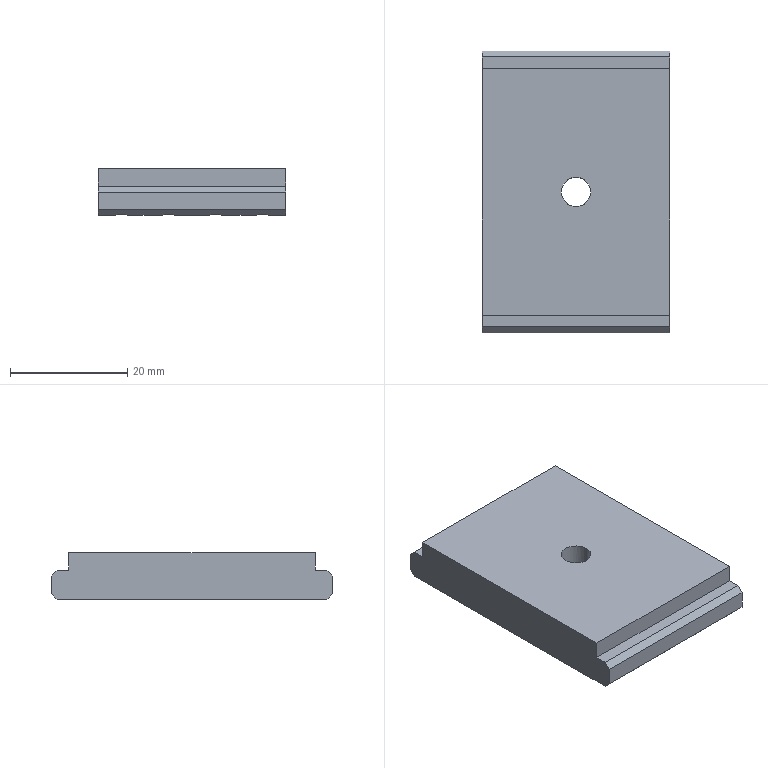Part | SolidWorks | features BaseBody 1, HoleWzd 1 | 1 solid | 43 faces | box 32 x 48 x 8 mm | volume 8228 mm3 | plane 33 | cylinder 10 | commonest cylinder face diameters 4.5 x8 5 x2
STEP:
#1=CARTESIAN_POINT('',(-1.75,-1.785,4.));
#2=VERTEX_POINT('',#1);
#3=CARTESIAN_POINT('',(-2.5,0.,4.));
#4=VERTEX_POINT('',#3);
#5=CARTESIAN_POINT('',(0.,0.,4.));
#6=DIRECTION('',(0.,0.,-1.));
#7=DIRECTION('',(-1.,0.,0.));
#8=AXIS2_PLACEMENT_3D('',#5,#6,#7);
#9=CIRCLE('',#8,2.5);
#10=EDGE_CURVE('',#2,#4,#9,.T.);
#11=ORIENTED_EDGE('',*,*,#10,.T.);
#12=CARTESIAN_POINT('',(-2.5,0.,8.));
#13=VERTEX_POINT('',#12);
#14=CARTESIAN_POINT('',(-2.5,0.,8.));
#15=DIRECTION('',(0.,0.,1.));
#16=VECTOR('',#15,1000.);
#17=LINE('',#14,#16);
#18=EDGE_CURVE('',#4,#13,#17,.T.);
#19=ORIENTED_EDGE('',*,*,#18,.T.);
#20=CARTESIAN_POINT('',(2.5,0.,8.));
#21=VERTEX_POINT('',#20);
#22=CARTESIAN_POINT('',(0.,0.,8.));
#23=DIRECTION('',(0.,0.,1.));
#24=DIRECTION('',(1.,0.,0.));
#25=AXIS2_PLACEMENT_3D('',#22,#23,#24);
#26=CIRCLE('',#25,2.5);
#27=EDGE_CURVE('',#13,#21,#26,.T.);
#28=ORIENTED_EDGE('',*,*,#27,.T.);
#29=CARTESIAN_POINT('',(2.5,0.,4.));
#30=VERTEX_POINT('',#29);
#31=CARTESIAN_POINT('',(2.5,0.,8.));
#32=DIRECTION('',(0.,0.,1.));
#33=VECTOR('',#32,1000.);
#34=LINE('',#31,#33);
#35=EDGE_CURVE('',#30,#21,#34,.T.);
#36=ORIENTED_EDGE('',*,*,#35,.F.);
#37=CARTESIAN_POINT('',(1.75,-1.785,4.));
#38=VERTEX_POINT('',#37);
#39=CARTESIAN_POINT('',(0.,0.,4.));
#40=DIRECTION('',(0.,0.,-1.));
#41=DIRECTION('',(-1.,0.,0.));
#42=AXIS2_PLACEMENT_3D('',#39,#40,#41);
#43=CIRCLE('',#42,2.5);
#44=EDGE_CURVE('',#30,#38,#43,.T.);
#45=ORIENTED_EDGE('',*,*,#44,.T.);
#46=CARTESIAN_POINT('',(1.75,-1.785,0.));
#47=VERTEX_POINT('',#46);
#48=CARTESIAN_POINT('',(1.75,-1.785,8.));
#49=DIRECTION('',(0.,0.,-1.));
#50=VECTOR('',#49,1000.);
#51=LINE('',#48,#50);
#52=EDGE_CURVE('',#38,#47,#51,.T.);
#53=ORIENTED_EDGE('',*,*,#52,.T.);
#54=CARTESIAN_POINT('',(-1.75,-1.785,0.));
#55=VERTEX_POINT('',#54);
#56=CARTESIAN_POINT('',(0.,0.,0.));
#57=DIRECTION('',(0.,0.,1.));
#58=DIRECTION('',(1.,0.,0.));
#59=AXIS2_PLACEMENT_3D('',#56,#57,#58);
#60=CIRCLE('',#59,2.5);
#61=EDGE_CURVE('',#55,#47,#60,.T.);
#62=ORIENTED_EDGE('',*,*,#61,.F.);
#63=CARTESIAN_POINT('',(-1.75,-1.785,8.));
#64=DIRECTION('',(0.,0.,-1.));
#65=VECTOR('',#64,1000.);
#66=LINE('',#63,#65);
#67=EDGE_CURVE('',#2,#55,#66,.T.);
#68=ORIENTED_EDGE('',*,*,#67,.F.);
#69=EDGE_LOOP('',(#11,#19,#28,#36,#45,#53,#62,#68));
#70=FACE_OUTER_BOUND('',#69,.T.);
#71=CARTESIAN_POINT('',(0.,0.,8.));
#72=DIRECTION('',(0.,0.,1.));
#73=DIRECTION('',(1.,0.,0.));
#74=AXIS2_PLACEMENT_3D('',#71,#72,#73);
#75=CYLINDRICAL_SURFACE('',#74,2.5);
#76=ADVANCED_FACE('',(#70),#75,.F.);
#77=CARTESIAN_POINT('',(1.75,1.785,0.));
#78=VERTEX_POINT('',#77);
#79=CARTESIAN_POINT('',(1.75,1.785,4.));
#80=VERTEX_POINT('',#79);
#81=CARTESIAN_POINT('',(1.75,1.785,8.));
#82=DIRECTION('',(0.,0.,1.));
#83=VECTOR('',#82,1000.);
#84=LINE('',#81,#83);
#85=EDGE_CURVE('',#78,#80,#84,.T.);
#86=ORIENTED_EDGE('',*,*,#85,.F.);
#87=CARTESIAN_POINT('',(1.75,21.,0.));
#88=VERTEX_POINT('',#87);
#89=CARTESIAN_POINT('',(1.75,21.,0.));
#90=DIRECTION('',(0.,-1.,0.));
#91=VECTOR('',#90,1000.);
#92=LINE('',#89,#91);
#93=EDGE_CURVE('',#88,#78,#92,.T.);
#94=ORIENTED_EDGE('',*,*,#93,.F.);
#95=CARTESIAN_POINT('',(1.75,21.,4.));
#96=VERTEX_POINT('',#95);
#97=CARTESIAN_POINT('',(1.75,21.,4.));
#98=DIRECTION('',(0.,0.,-1.));
#99=VECTOR('',#98,1000.);
#100=LINE('',#97,#99);
#101=EDGE_CURVE('',#96,#88,#100,.T.);
#102=ORIENTED_EDGE('',*,*,#101,.F.);
#103=CARTESIAN_POINT('',(1.75,21.,4.));
#104=DIRECTION('',(0.,-1.,0.));
#105=VECTOR('',#104,1000.);
#106=LINE('',#103,#105);
#107=EDGE_CURVE('',#96,#80,#106,.T.);
#108=ORIENTED_EDGE('',*,*,#107,.T.);
#109=EDGE_LOOP('',(#86,#94,#102,#108));
#110=FACE_OUTER_BOUND('',#109,.T.);
#111=CARTESIAN_POINT('',(1.75,21.,4.));
#112=DIRECTION('',(1.,0.,0.));
#113=DIRECTION('',(0.,1.,0.));
#114=AXIS2_PLACEMENT_3D('',#111,#112,#113);
#115=PLANE('',#114);
#116=ADVANCED_FACE('',(#110),#115,.T.);
#117=ORIENTED_EDGE('',*,*,#93,.T.);
#118=CARTESIAN_POINT('',(-1.75,1.785,0.));
#119=VERTEX_POINT('',#118);
#120=CARTESIAN_POINT('',(0.,0.,0.));
#121=DIRECTION('',(0.,0.,1.));
#122=DIRECTION('',(1.,0.,0.));
#123=AXIS2_PLACEMENT_3D('',#120,#121,#122);
#124=CIRCLE('',#123,2.5);
#125=EDGE_CURVE('',#78,#119,#124,.T.);
#126=ORIENTED_EDGE('',*,*,#125,.T.);
#127=CARTESIAN_POINT('',(-1.75,21.,0.));
#128=VERTEX_POINT('',#127);
#129=CARTESIAN_POINT('',(-1.75,21.,0.));
#130=DIRECTION('',(0.,-1.,0.));
#131=VECTOR('',#130,1000.);
#132=LINE('',#129,#131);
#133=EDGE_CURVE('',#128,#119,#132,.T.);
#134=ORIENTED_EDGE('',*,*,#133,.F.);
#135=CARTESIAN_POINT('',(-2.969,23.,0.));
#136=VERTEX_POINT('',#135);
#137=CARTESIAN_POINT('',(-4.,21.,0.));
#138=DIRECTION('',(0.,0.,-1.));
#139=DIRECTION('',(-1.,0.,0.));
#140=AXIS2_PLACEMENT_3D('',#137,#138,#139);
#141=CIRCLE('',#140,2.25);
#142=EDGE_CURVE('',#136,#128,#141,.T.);
#143=ORIENTED_EDGE('',*,*,#142,.F.);
#144=CARTESIAN_POINT('',(2.969,23.,0.));
#145=VERTEX_POINT('',#144);
#146=CARTESIAN_POINT('',(0.,23.,0.));
#147=DIRECTION('',(1.,0.,0.));
#148=VECTOR('',#147,1000.);
#149=LINE('',#146,#148);
#150=EDGE_CURVE('',#136,#145,#149,.T.);
#151=ORIENTED_EDGE('',*,*,#150,.T.);
#152=CARTESIAN_POINT('',(4.,21.,0.));
#153=DIRECTION('',(0.,0.,1.));
#154=DIRECTION('',(1.,0.,0.));
#155=AXIS2_PLACEMENT_3D('',#152,#153,#154);
#156=CIRCLE('',#155,2.25);
#157=EDGE_CURVE('',#145,#88,#156,.T.);
#158=ORIENTED_EDGE('',*,*,#157,.T.);
#159=EDGE_LOOP('',(#117,#126,#134,#143,#151,#158));
#160=FACE_OUTER_BOUND('',#159,.T.);
#161=CARTESIAN_POINT('',(0.,0.,0.));
#162=DIRECTION('',(0.,0.,1.));
#163=DIRECTION('',(1.,0.,0.));
#164=AXIS2_PLACEMENT_3D('',#161,#162,#163);
#165=PLANE('',#164);
#166=ADVANCED_FACE('',(#160),#165,.F.);
#167=ORIENTED_EDGE('',*,*,#133,.T.);
#168=CARTESIAN_POINT('',(-1.75,1.785,4.));
#169=VERTEX_POINT('',#168);
#170=CARTESIAN_POINT('',(-1.75,1.785,8.));
#171=DIRECTION('',(0.,0.,1.));
#172=VECTOR('',#171,1000.);
#173=LINE('',#170,#172);
#174=EDGE_CURVE('',#119,#169,#173,.T.);
#175=ORIENTED_EDGE('',*,*,#174,.T.);
#176=CARTESIAN_POINT('',(-1.75,21.,4.));
#177=VERTEX_POINT('',#176);
#178=CARTESIAN_POINT('',(-1.75,21.,4.));
#179=DIRECTION('',(0.,-1.,0.));
#180=VECTOR('',#179,1000.);
#181=LINE('',#178,#180);
#182=EDGE_CURVE('',#177,#169,#181,.T.);
#183=ORIENTED_EDGE('',*,*,#182,.F.);
#184=CARTESIAN_POINT('',(-1.75,21.,4.));
#185=DIRECTION('',(0.,0.,-1.));
#186=VECTOR('',#185,1000.);
#187=LINE('',#184,#186);
#188=EDGE_CURVE('',#177,#128,#187,.T.);
#189=ORIENTED_EDGE('',*,*,#188,.T.);
#190=EDGE_LOOP('',(#167,#175,#183,#189));
#191=FACE_OUTER_BOUND('',#190,.T.);
#192=CARTESIAN_POINT('',(-1.75,21.,4.));
#193=DIRECTION('',(1.,0.,0.));
#194=DIRECTION('',(0.,1.,0.));
#195=AXIS2_PLACEMENT_3D('',#192,#193,#194);
#196=PLANE('',#195);
#197=ADVANCED_FACE('',(#191),#196,.F.);
#198=CARTESIAN_POINT('',(13.031,-23.,0.));
#199=VERTEX_POINT('',#198);
#200=CARTESIAN_POINT('',(10.969,-23.,0.));
#201=VERTEX_POINT('',#200);
#202=CARTESIAN_POINT('',(13.031,-23.,0.));
#203=CARTESIAN_POINT('',(12.371,-23.34,0.34));
#204=CARTESIAN_POINT('',(11.629,-23.34,0.34));
#205=CARTESIAN_POINT('',(10.969,-23.,0.));
#206=(BOUNDED_CURVE()B_SPLINE_CURVE(3,(#202,#203,#204,#205),.UNSPECIFIED.,.F.,.F.)B_SPLINE_CURVE_WITH_KNOTS((4,4),(2.666,3.617),.UNSPECIFIED.)CURVE()GEOMETRIC_REPRESENTATION_ITEM()RATIONAL_B_SPLINE_CURVE((1.,0.9259,0.9259,1.))REPRESENTATION_ITEM(''));
#207=EDGE_CURVE('',#199,#201,#206,.T.);
#208=ORIENTED_EDGE('',*,*,#207,.F.);
#209=CARTESIAN_POINT('',(16.,-23.,0.));
#210=VERTEX_POINT('',#209);
#211=CARTESIAN_POINT('',(0.,-23.,0.));
#212=DIRECTION('',(-1.,0.,0.));
#213=VECTOR('',#212,1000.);
#214=LINE('',#211,#213);
#215=EDGE_CURVE('',#210,#199,#214,.T.);
#216=ORIENTED_EDGE('',*,*,#215,.F.);
#217=CARTESIAN_POINT('',(16.,-24.,1.));
#218=VERTEX_POINT('',#217);
#219=CARTESIAN_POINT('',(16.,-24.,1.));
#220=DIRECTION('',(0.,0.7071,-0.7071));
#221=VECTOR('',#220,1000.);
#222=LINE('',#219,#221);
#223=EDGE_CURVE('',#218,#210,#222,.T.);
#224=ORIENTED_EDGE('',*,*,#223,.F.);
#225=CARTESIAN_POINT('',(-16.,-24.,1.));
#226=VERTEX_POINT('',#225);
#227=CARTESIAN_POINT('',(-16.,-24.,1.));
#228=DIRECTION('',(1.,0.,0.));
#229=VECTOR('',#228,1000.);
#230=LINE('',#227,#229);
#231=EDGE_CURVE('',#226,#218,#230,.T.);
#232=ORIENTED_EDGE('',*,*,#231,.F.);
#233=CARTESIAN_POINT('',(-16.,-23.,0.));
#234=VERTEX_POINT('',#233);
#235=CARTESIAN_POINT('',(-16.,-24.,1.));
#236=DIRECTION('',(0.,-0.7071,0.7071));
#237=VECTOR('',#236,1000.);
#238=LINE('',#235,#237);
#239=EDGE_CURVE('',#234,#226,#238,.T.);
#240=ORIENTED_EDGE('',*,*,#239,.F.);
#241=CARTESIAN_POINT('',(-13.031,-23.,0.));
#242=VERTEX_POINT('',#241);
#243=CARTESIAN_POINT('',(0.,-23.,0.));
#244=DIRECTION('',(-1.,0.,0.));
#245=VECTOR('',#244,1000.);
#246=LINE('',#243,#245);
#247=EDGE_CURVE('',#242,#234,#246,.T.);
#248=ORIENTED_EDGE('',*,*,#247,.F.);
#249=CARTESIAN_POINT('',(-10.969,-23.,0.));
#250=VERTEX_POINT('',#249);
#251=CARTESIAN_POINT('',(-10.969,-23.,0.));
#252=CARTESIAN_POINT('',(-11.629,-23.34,0.34));
#253=CARTESIAN_POINT('',(-12.371,-23.34,0.34));
#254=CARTESIAN_POINT('',(-13.031,-23.,0.));
#255=(BOUNDED_CURVE()B_SPLINE_CURVE(3,(#251,#252,#253,#254),.UNSPECIFIED.,.F.,.T.)B_SPLINE_CURVE_WITH_KNOTS((4,4),(2.666,3.617),.UNSPECIFIED.)CURVE()GEOMETRIC_REPRESENTATION_ITEM()RATIONAL_B_SPLINE_CURVE((1.,0.9259,0.9259,1.))REPRESENTATION_ITEM(''));
#256=EDGE_CURVE('',#250,#242,#255,.T.);
#257=ORIENTED_EDGE('',*,*,#256,.F.);
#258=CARTESIAN_POINT('',(-5.031,-23.,0.));
#259=VERTEX_POINT('',#258);
#260=CARTESIAN_POINT('',(0.,-23.,0.));
#261=DIRECTION('',(-1.,0.,0.));
#262=VECTOR('',#261,1000.);
#263=LINE('',#260,#262);
#264=EDGE_CURVE('',#259,#250,#263,.T.);
#265=ORIENTED_EDGE('',*,*,#264,.F.);
#266=CARTESIAN_POINT('',(-2.969,-23.,0.));
#267=VERTEX_POINT('',#266);
#268=CARTESIAN_POINT('',(-2.969,-23.,0.));
#269=CARTESIAN_POINT('',(-3.629,-23.34,0.34));
#270=CARTESIAN_POINT('',(-4.371,-23.34,0.34));
#271=CARTESIAN_POINT('',(-5.031,-23.,0.));
#272=(BOUNDED_CURVE()B_SPLINE_CURVE(3,(#268,#269,#270,#271),.UNSPECIFIED.,.F.,.F.)B_SPLINE_CURVE_WITH_KNOTS((4,4),(2.666,3.617),.UNSPECIFIED.)CURVE()GEOMETRIC_REPRESENTATION_ITEM()RATIONAL_B_SPLINE_CURVE((1.,0.9259,0.9259,1.))REPRESENTATION_ITEM(''));
#273=EDGE_CURVE('',#267,#259,#272,.T.);
#274=ORIENTED_EDGE('',*,*,#273,.F.);
#275=CARTESIAN_POINT('',(2.969,-23.,0.));
#276=VERTEX_POINT('',#275);
#277=CARTESIAN_POINT('',(0.,-23.,0.));
#278=DIRECTION('',(-1.,0.,0.));
#279=VECTOR('',#278,1000.);
#280=LINE('',#277,#279);
#281=EDGE_CURVE('',#276,#267,#280,.T.);
#282=ORIENTED_EDGE('',*,*,#281,.F.);
#283=CARTESIAN_POINT('',(5.031,-23.,0.));
#284=VERTEX_POINT('',#283);
#285=CARTESIAN_POINT('',(5.031,-23.,0.));
#286=CARTESIAN_POINT('',(4.371,-23.34,0.34));
#287=CARTESIAN_POINT('',(3.629,-23.34,0.34));
#288=CARTESIAN_POINT('',(2.969,-23.,0.));
#289=(BOUNDED_CURVE()B_SPLINE_CURVE(3,(#285,#286,#287,#288),.UNSPECIFIED.,.F.,.F.)B_SPLINE_CURVE_WITH_KNOTS((4,4),(2.666,3.617),.UNSPECIFIED.)CURVE()GEOMETRIC_REPRESENTATION_ITEM()RATIONAL_B_SPLINE_CURVE((1.,0.9259,0.9259,1.))REPRESENTATION_ITEM(''));
#290=EDGE_CURVE('',#284,#276,#289,.T.);
#291=ORIENTED_EDGE('',*,*,#290,.F.);
#292=CARTESIAN_POINT('',(0.,-23.,0.));
#293=DIRECTION('',(-1.,0.,0.));
#294=VECTOR('',#293,1000.);
#295=LINE('',#292,#294);
#296=EDGE_CURVE('',#201,#284,#295,.T.);
#297=ORIENTED_EDGE('',*,*,#296,.F.);
#298=EDGE_LOOP('',(#208,#216,#224,#232,#240,#248,#257,#265,#274,#282,#291,#297));
#299=FACE_OUTER_BOUND('',#298,.T.);
#300=CARTESIAN_POINT('',(-16.,-24.,1.));
#301=DIRECTION('',(0.,0.7071,0.7071));
#302=DIRECTION('',(1.,0.,0.));
#303=AXIS2_PLACEMENT_3D('',#300,#301,#302);
#304=PLANE('',#303);
#305=ADVANCED_FACE('',(#299),#304,.F.);
#306=CARTESIAN_POINT('',(-16.,-24.,4.));
#307=VERTEX_POINT('',#306);
#308=CARTESIAN_POINT('',(-16.,-23.,5.));
#309=VERTEX_POINT('',#308);
#310=CARTESIAN_POINT('',(-16.,-23.,5.));
#311=DIRECTION('',(0.,0.7071,0.7071));
#312=VECTOR('',#311,1000.);
#313=LINE('',#310,#312);
#314=EDGE_CURVE('',#307,#309,#313,.T.);
#315=ORIENTED_EDGE('',*,*,#314,.F.);
#316=CARTESIAN_POINT('',(16.,-24.,4.));
#317=VERTEX_POINT('',#316);
#318=CARTESIAN_POINT('',(-16.,-24.,4.));
#319=DIRECTION('',(-1.,0.,0.));
#320=VECTOR('',#319,1000.);
#321=LINE('',#318,#320);
#322=EDGE_CURVE('',#317,#307,#321,.T.);
#323=ORIENTED_EDGE('',*,*,#322,.F.);
#324=CARTESIAN_POINT('',(16.,-23.,5.));
#325=VERTEX_POINT('',#324);
#326=CARTESIAN_POINT('',(16.,-23.,5.));
#327=DIRECTION('',(0.,-0.7071,-0.7071));
#328=VECTOR('',#327,1000.);
#329=LINE('',#326,#328);
#330=EDGE_CURVE('',#325,#317,#329,.T.);
#331=ORIENTED_EDGE('',*,*,#330,.F.);
#332=CARTESIAN_POINT('',(-23.,-23.,5.));
#333=DIRECTION('',(1.,0.,0.));
#334=VECTOR('',#333,1000.);
#335=LINE('',#332,#334);
#336=EDGE_CURVE('',#309,#325,#335,.T.);
#337=ORIENTED_EDGE('',*,*,#336,.F.);
#338=EDGE_LOOP('',(#315,#323,#331,#337));
#339=FACE_OUTER_BOUND('',#338,.T.);
#340=CARTESIAN_POINT('',(-23.,-23.,5.));
#341=DIRECTION('',(0.,0.7071,-0.7071));
#342=DIRECTION('',(-1.,0.,0.));
#343=AXIS2_PLACEMENT_3D('',#340,#341,#342);
#344=PLANE('',#343);
#345=ADVANCED_FACE('',(#339),#344,.F.);
#346=CARTESIAN_POINT('',(-13.031,23.,0.));
#347=VERTEX_POINT('',#346);
#348=CARTESIAN_POINT('',(-10.969,23.,0.));
#349=VERTEX_POINT('',#348);
#350=CARTESIAN_POINT('',(-13.031,23.,0.));
#351=CARTESIAN_POINT('',(-12.371,23.34,0.34));
#352=CARTESIAN_POINT('',(-11.629,23.34,0.34));
#353=CARTESIAN_POINT('',(-10.969,23.,0.));
#354=(BOUNDED_CURVE()B_SPLINE_CURVE(3,(#350,#351,#352,#353),.UNSPECIFIED.,.F.,.F.)B_SPLINE_CURVE_WITH_KNOTS((4,4),(5.807,6.759),.UNSPECIFIED.)CURVE()GEOMETRIC_REPRESENTATION_ITEM()RATIONAL_B_SPLINE_CURVE((1.,0.9259,0.9259,1.))REPRESENTATION_ITEM(''));
#355=EDGE_CURVE('',#347,#349,#354,.T.);
#356=ORIENTED_EDGE('',*,*,#355,.F.);
#357=CARTESIAN_POINT('',(-16.,23.,0.));
#358=VERTEX_POINT('',#357);
#359=CARTESIAN_POINT('',(0.,23.,0.));
#360=DIRECTION('',(1.,0.,0.));
#361=VECTOR('',#360,1000.);
#362=LINE('',#359,#361);
#363=EDGE_CURVE('',#358,#347,#362,.T.);
#364=ORIENTED_EDGE('',*,*,#363,.F.);
#365=CARTESIAN_POINT('',(-16.,24.,1.));
#366=VERTEX_POINT('',#365);
#367=CARTESIAN_POINT('',(-16.,24.,1.));
#368=DIRECTION('',(0.,-0.7071,-0.7071));
#369=VECTOR('',#368,1000.);
#370=LINE('',#367,#369);
#371=EDGE_CURVE('',#366,#358,#370,.T.);
#372=ORIENTED_EDGE('',*,*,#371,.F.);
#373=CARTESIAN_POINT('',(16.,24.,1.));
#374=VERTEX_POINT('',#373);
#375=CARTESIAN_POINT('',(-16.,24.,1.));
#376=DIRECTION('',(-1.,0.,0.));
#377=VECTOR('',#376,1000.);
#378=LINE('',#375,#377);
#379=EDGE_CURVE('',#374,#366,#378,.T.);
#380=ORIENTED_EDGE('',*,*,#379,.F.);
#381=CARTESIAN_POINT('',(16.,23.,0.));
#382=VERTEX_POINT('',#381);
#383=CARTESIAN_POINT('',(16.,24.,1.));
#384=DIRECTION('',(0.,0.7071,0.7071));
#385=VECTOR('',#384,1000.);
#386=LINE('',#383,#385);
#387=EDGE_CURVE('',#382,#374,#386,.T.);
#388=ORIENTED_EDGE('',*,*,#387,.F.);
#389=CARTESIAN_POINT('',(13.031,23.,0.));
#390=VERTEX_POINT('',#389);
#391=CARTESIAN_POINT('',(0.,23.,0.));
#392=DIRECTION('',(1.,0.,0.));
#393=VECTOR('',#392,1000.);
#394=LINE('',#391,#393);
#395=EDGE_CURVE('',#390,#382,#394,.T.);
#396=ORIENTED_EDGE('',*,*,#395,.F.);
#397=CARTESIAN_POINT('',(10.969,23.,0.));
#398=VERTEX_POINT('',#397);
#399=CARTESIAN_POINT('',(10.969,23.,0.));
#400=CARTESIAN_POINT('',(11.629,23.34,0.34));
#401=CARTESIAN_POINT('',(12.371,23.34,0.34));
#402=CARTESIAN_POINT('',(13.031,23.,0.));
#403=(BOUNDED_CURVE()B_SPLINE_CURVE(3,(#399,#400,#401,#402),.UNSPECIFIED.,.F.,.F.)B_SPLINE_CURVE_WITH_KNOTS((4,4),(5.807,6.759),.UNSPECIFIED.)CURVE()GEOMETRIC_REPRESENTATION_ITEM()RATIONAL_B_SPLINE_CURVE((1.,0.9259,0.9259,1.))REPRESENTATION_ITEM(''));
#404=EDGE_CURVE('',#398,#390,#403,.T.);
#405=ORIENTED_EDGE('',*,*,#404,.F.);
#406=CARTESIAN_POINT('',(5.031,23.,0.));
#407=VERTEX_POINT('',#406);
#408=CARTESIAN_POINT('',(0.,23.,0.));
#409=DIRECTION('',(1.,0.,0.));
#410=VECTOR('',#409,1000.);
#411=LINE('',#408,#410);
#412=EDGE_CURVE('',#407,#398,#411,.T.);
#413=ORIENTED_EDGE('',*,*,#412,.F.);
#414=CARTESIAN_POINT('',(2.969,23.,0.));
#415=CARTESIAN_POINT('',(3.629,23.34,0.34));
#416=CARTESIAN_POINT('',(4.371,23.34,0.34));
#417=CARTESIAN_POINT('',(5.031,23.,0.));
#418=(BOUNDED_CURVE()B_SPLINE_CURVE(3,(#414,#415,#416,#417),.UNSPECIFIED.,.F.,.F.)B_SPLINE_CURVE_WITH_KNOTS((4,4),(5.807,6.759),.UNSPECIFIED.)CURVE()GEOMETRIC_REPRESENTATION_ITEM()RATIONAL_B_SPLINE_CURVE((1.,0.9259,0.9259,1.))REPRESENTATION_ITEM(''));
#419=EDGE_CURVE('',#145,#407,#418,.T.);
#420=ORIENTED_EDGE('',*,*,#419,.F.);
#421=ORIENTED_EDGE('',*,*,#150,.F.);
#422=CARTESIAN_POINT('',(-5.031,23.,0.));
#423=VERTEX_POINT('',#422);
#424=CARTESIAN_POINT('',(-5.031,23.,0.));
#425=CARTESIAN_POINT('',(-4.371,23.34,0.34));
#426=CARTESIAN_POINT('',(-3.629,23.34,0.34));
#427=CARTESIAN_POINT('',(-2.969,23.,0.));
#428=(BOUNDED_CURVE()B_SPLINE_CURVE(3,(#424,#425,#426,#427),.UNSPECIFIED.,.F.,.F.)B_SPLINE_CURVE_WITH_KNOTS((4,4),(5.807,6.759),.UNSPECIFIED.)CURVE()GEOMETRIC_REPRESENTATION_ITEM()RATIONAL_B_SPLINE_CURVE((1.,0.9259,0.9259,1.))REPRESENTATION_ITEM(''));
#429=EDGE_CURVE('',#423,#136,#428,.T.);
#430=ORIENTED_EDGE('',*,*,#429,.F.);
#431=CARTESIAN_POINT('',(0.,23.,0.));
#432=DIRECTION('',(1.,0.,0.));
#433=VECTOR('',#432,1000.);
#434=LINE('',#431,#433);
#435=EDGE_CURVE('',#349,#423,#434,.T.);
#436=ORIENTED_EDGE('',*,*,#435,.F.);
#437=EDGE_LOOP('',(#356,#364,#372,#380,#388,#396,#405,#413,#420,#421,#430,#436));
#438=FACE_OUTER_BOUND('',#437,.T.);
#439=CARTESIAN_POINT('',(-16.,24.,1.));
#440=DIRECTION('',(0.,-0.7071,0.7071));
#441=DIRECTION('',(-1.,0.,0.));
#442=AXIS2_PLACEMENT_3D('',#439,#440,#441);
#443=PLANE('',#442);
#444=ADVANCED_FACE('',(#438),#443,.F.);
#445=CARTESIAN_POINT('',(-16.,23.,5.));
#446=VERTEX_POINT('',#445);
#447=CARTESIAN_POINT('',(-16.,24.,4.));
#448=VERTEX_POINT('',#447);
#449=CARTESIAN_POINT('',(-16.,24.,4.));
#450=DIRECTION('',(0.,0.7071,-0.7071));
#451=VECTOR('',#450,1000.);
#452=LINE('',#449,#451);
#453=EDGE_CURVE('',#446,#448,#452,.T.);
#454=ORIENTED_EDGE('',*,*,#453,.F.);
#455=CARTESIAN_POINT('',(16.,23.,5.));
#456=VERTEX_POINT('',#455);
#457=CARTESIAN_POINT('',(-23.,23.,5.));
#458=DIRECTION('',(-1.,0.,0.));
#459=VECTOR('',#458,1000.);
#460=LINE('',#457,#459);
#461=EDGE_CURVE('',#456,#446,#460,.T.);
#462=ORIENTED_EDGE('',*,*,#461,.F.);
#463=CARTESIAN_POINT('',(16.,24.,4.));
#464=VERTEX_POINT('',#463);
#465=CARTESIAN_POINT('',(16.,24.,4.));
#466=DIRECTION('',(0.,-0.7071,0.7071));
#467=VECTOR('',#466,1000.);
#468=LINE('',#465,#467);
#469=EDGE_CURVE('',#464,#456,#468,.T.);
#470=ORIENTED_EDGE('',*,*,#469,.F.);
#471=CARTESIAN_POINT('',(-16.,24.,4.));
#472=DIRECTION('',(1.,0.,0.));
#473=VECTOR('',#472,1000.);
#474=LINE('',#471,#473);
#475=EDGE_CURVE('',#448,#464,#474,.T.);
#476=ORIENTED_EDGE('',*,*,#475,.F.);
#477=EDGE_LOOP('',(#454,#462,#470,#476));
#478=FACE_OUTER_BOUND('',#477,.T.);
#479=CARTESIAN_POINT('',(-16.,24.,4.));
#480=DIRECTION('',(0.,-0.7071,-0.7071));
#481=DIRECTION('',(0.,-0.7071,0.7071));
#482=AXIS2_PLACEMENT_3D('',#479,#480,#481);
#483=PLANE('',#482);
#484=ADVANCED_FACE('',(#478),#483,.F.);
#485=CARTESIAN_POINT('',(-16.,21.,8.));
#486=VERTEX_POINT('',#485);
#487=CARTESIAN_POINT('',(16.,21.,8.));
#488=VERTEX_POINT('',#487);
#489=CARTESIAN_POINT('',(0.,21.,8.));
#490=DIRECTION('',(1.,0.,0.));
#491=VECTOR('',#490,1000.);
#492=LINE('',#489,#491);
#493=EDGE_CURVE('',#486,#488,#492,.T.);
#494=ORIENTED_EDGE('',*,*,#493,.T.);
#495=CARTESIAN_POINT('',(16.,21.,5.));
#496=VERTEX_POINT('',#495);
#497=CARTESIAN_POINT('',(16.,21.,8.));
#498=DIRECTION('',(0.,0.,-1.));
#499=VECTOR('',#498,1000.);
#500=LINE('',#497,#499);
#501=EDGE_CURVE('',#488,#496,#500,.T.);
#502=ORIENTED_EDGE('',*,*,#501,.T.);
#503=CARTESIAN_POINT('',(-16.,21.,5.));
#504=VERTEX_POINT('',#503);
#505=CARTESIAN_POINT('',(-23.,21.,5.));
#506=DIRECTION('',(1.,0.,0.));
#507=VECTOR('',#506,1000.);
#508=LINE('',#505,#507);
#509=EDGE_CURVE('',#504,#496,#508,.T.);
#510=ORIENTED_EDGE('',*,*,#509,.F.);
#511=CARTESIAN_POINT('',(-16.,21.,8.));
#512=DIRECTION('',(0.,0.,-1.));
#513=VECTOR('',#512,1000.);
#514=LINE('',#511,#513);
#515=EDGE_CURVE('',#486,#504,#514,.T.);
#516=ORIENTED_EDGE('',*,*,#515,.F.);
#517=EDGE_LOOP('',(#494,#502,#510,#516));
#518=FACE_OUTER_BOUND('',#517,.T.);
#519=CARTESIAN_POINT('',(-23.,21.,8.));
#520=DIRECTION('',(0.,-1.,0.));
#521=DIRECTION('',(0.,0.,-1.));
#522=AXIS2_PLACEMENT_3D('',#519,#520,#521);
#523=PLANE('',#522);
#524=ADVANCED_FACE('',(#518),#523,.F.);
#525=CARTESIAN_POINT('',(16.,24.,5.));
#526=DIRECTION('',(0.,1.,0.));
#527=VECTOR('',#526,1000.);
#528=LINE('',#525,#527);
#529=EDGE_CURVE('',#496,#456,#528,.T.);
#530=ORIENTED_EDGE('',*,*,#529,.T.);
#531=ORIENTED_EDGE('',*,*,#461,.T.);
#532=CARTESIAN_POINT('',(-16.,24.,5.));
#533=DIRECTION('',(0.,1.,0.));
#534=VECTOR('',#533,1000.);
#535=LINE('',#532,#534);
#536=EDGE_CURVE('',#504,#446,#535,.T.);
#537=ORIENTED_EDGE('',*,*,#536,.F.);
#538=ORIENTED_EDGE('',*,*,#509,.T.);
#539=EDGE_LOOP('',(#530,#531,#537,#538));
#540=FACE_OUTER_BOUND('',#539,.T.);
#541=CARTESIAN_POINT('',(-23.,24.,5.));
#542=DIRECTION('',(0.,0.,-1.));
#543=DIRECTION('',(0.,-1.,0.));
#544=AXIS2_PLACEMENT_3D('',#541,#542,#543);
#545=PLANE('',#544);
#546=ADVANCED_FACE('',(#540),#545,.F.);
#547=CARTESIAN_POINT('',(-16.,-21.,5.));
#548=VERTEX_POINT('',#547);
#549=CARTESIAN_POINT('',(16.,-21.,5.));
#550=VERTEX_POINT('',#549);
#551=CARTESIAN_POINT('',(-23.,-21.,5.));
#552=DIRECTION('',(1.,0.,0.));
#553=VECTOR('',#552,1000.);
#554=LINE('',#551,#553);
#555=EDGE_CURVE('',#548,#550,#554,.T.);
#556=ORIENTED_EDGE('',*,*,#555,.T.);
#557=CARTESIAN_POINT('',(16.,-21.,8.));
#558=VERTEX_POINT('',#557);
#559=CARTESIAN_POINT('',(16.,-21.,8.));
#560=DIRECTION('',(0.,0.,1.));
#561=VECTOR('',#560,1000.);
#562=LINE('',#559,#561);
#563=EDGE_CURVE('',#550,#558,#562,.T.);
#564=ORIENTED_EDGE('',*,*,#563,.T.);
#565=CARTESIAN_POINT('',(-16.,-21.,8.));
#566=VERTEX_POINT('',#565);
#567=CARTESIAN_POINT('',(0.,-21.,8.));
#568=DIRECTION('',(-1.,0.,0.));
#569=VECTOR('',#568,1000.);
#570=LINE('',#567,#569);
#571=EDGE_CURVE('',#558,#566,#570,.T.);
#572=ORIENTED_EDGE('',*,*,#571,.T.);
#573=CARTESIAN_POINT('',(-16.,-21.,8.));
#574=DIRECTION('',(0.,0.,1.));
#575=VECTOR('',#574,1000.);
#576=LINE('',#573,#575);
#577=EDGE_CURVE('',#548,#566,#576,.T.);
#578=ORIENTED_EDGE('',*,*,#577,.F.);
#579=EDGE_LOOP('',(#556,#564,#572,#578));
#580=FACE_OUTER_BOUND('',#579,.T.);
#581=CARTESIAN_POINT('',(-23.,-21.,8.));
#582=DIRECTION('',(0.,1.,0.));
#583=DIRECTION('',(1.,0.,0.));
#584=AXIS2_PLACEMENT_3D('',#581,#582,#583);
#585=PLANE('',#584);
#586=ADVANCED_FACE('',(#580),#585,.F.);
#587=CARTESIAN_POINT('',(-16.,24.,5.));
#588=DIRECTION('',(0.,1.,0.));
#589=VECTOR('',#588,1000.);
#590=LINE('',#587,#589);
#591=EDGE_CURVE('',#309,#548,#590,.T.);
#592=ORIENTED_EDGE('',*,*,#591,.F.);
#593=ORIENTED_EDGE('',*,*,#336,.T.);
#594=CARTESIAN_POINT('',(16.,-24.,5.));
#595=DIRECTION('',(0.,1.,0.));
#596=VECTOR('',#595,1000.);
#597=LINE('',#594,#596);
#598=EDGE_CURVE('',#325,#550,#597,.T.);
#599=ORIENTED_EDGE('',*,*,#598,.T.);
#600=ORIENTED_EDGE('',*,*,#555,.F.);
#601=EDGE_LOOP('',(#592,#593,#599,#600));
#602=FACE_OUTER_BOUND('',#601,.T.);
#603=CARTESIAN_POINT('',(-23.,-24.,5.));
#604=DIRECTION('',(0.,0.,-1.));
#605=DIRECTION('',(0.,-1.,0.));
#606=AXIS2_PLACEMENT_3D('',#603,#604,#605);
#607=PLANE('',#606);
#608=ADVANCED_FACE('',(#602),#607,.F.);
#609=CARTESIAN_POINT('',(0.,0.,4.));
#610=DIRECTION('',(0.,0.,-1.));
#611=DIRECTION('',(-1.,0.,0.));
#612=AXIS2_PLACEMENT_3D('',#609,#610,#611);
#613=CIRCLE('',#612,2.5);
#614=EDGE_CURVE('',#80,#30,#613,.T.);
#615=ORIENTED_EDGE('',*,*,#614,.F.);
#616=ORIENTED_EDGE('',*,*,#107,.F.);
#617=CARTESIAN_POINT('',(6.25,21.,4.));
#618=VERTEX_POINT('',#617);
#619=CARTESIAN_POINT('',(4.,21.,4.));
#620=DIRECTION('',(0.,0.,1.));
#621=DIRECTION('',(1.,0.,0.));
#622=AXIS2_PLACEMENT_3D('',#619,#620,#621);
#623=CIRCLE('',#622,2.25);
#624=EDGE_CURVE('',#618,#96,#623,.T.);
#625=ORIENTED_EDGE('',*,*,#624,.F.);
#626=CARTESIAN_POINT('',(6.25,-21.,4.));
#627=VERTEX_POINT('',#626);
#628=CARTESIAN_POINT('',(6.25,21.,4.));
#629=DIRECTION('',(0.,1.,0.));
#630=VECTOR('',#629,1000.);
#631=LINE('',#628,#630);
#632=EDGE_CURVE('',#627,#618,#631,.T.);
#633=ORIENTED_EDGE('',*,*,#632,.F.);
#634=CARTESIAN_POINT('',(1.75,-21.,4.));
#635=VERTEX_POINT('',#634);
#636=CARTESIAN_POINT('',(4.,-21.,4.));
#637=DIRECTION('',(0.,0.,1.));
#638=DIRECTION('',(1.,0.,0.));
#639=AXIS2_PLACEMENT_3D('',#636,#637,#638);
#640=CIRCLE('',#639,2.25);
#641=EDGE_CURVE('',#635,#627,#640,.T.);
#642=ORIENTED_EDGE('',*,*,#641,.F.);
#643=CARTESIAN_POINT('',(1.75,21.,4.));
#644=DIRECTION('',(0.,-1.,0.));
#645=VECTOR('',#644,1000.);
#646=LINE('',#643,#645);
#647=EDGE_CURVE('',#38,#635,#646,.T.);
#648=ORIENTED_EDGE('',*,*,#647,.F.);
#649=ORIENTED_EDGE('',*,*,#44,.F.);
#650=EDGE_LOOP('',(#615,#616,#625,#633,#642,#648,#649));
#651=FACE_OUTER_BOUND('',#650,.T.);
#652=CARTESIAN_POINT('',(4.,21.,4.));
#653=DIRECTION('',(0.,0.,-1.));
#654=DIRECTION('',(0.,-1.,0.));
#655=AXIS2_PLACEMENT_3D('',#652,#653,#654);
#656=PLANE('',#655);
#657=ADVANCED_FACE('',(#651),#656,.T.);
#658=CARTESIAN_POINT('',(6.25,-21.,0.));
#659=VERTEX_POINT('',#658);
#660=CARTESIAN_POINT('',(6.25,21.,0.));
#661=VERTEX_POINT('',#660);
#662=CARTESIAN_POINT('',(6.25,21.,0.));
#663=DIRECTION('',(0.,1.,0.));
#664=VECTOR('',#663,1000.);
#665=LINE('',#662,#664);
#666=EDGE_CURVE('',#659,#661,#665,.T.);
#667=ORIENTED_EDGE('',*,*,#666,.F.);
#668=CARTESIAN_POINT('',(6.25,-21.,4.));
#669=DIRECTION('',(0.,0.,-1.));
#670=VECTOR('',#669,1000.);
#671=LINE('',#668,#670);
#672=EDGE_CURVE('',#627,#659,#671,.T.);
#673=ORIENTED_EDGE('',*,*,#672,.F.);
#674=ORIENTED_EDGE('',*,*,#632,.T.);
#675=CARTESIAN_POINT('',(6.25,21.,4.));
#676=DIRECTION('',(0.,0.,-1.));
#677=VECTOR('',#676,1000.);
#678=LINE('',#675,#677);
#679=EDGE_CURVE('',#618,#661,#678,.T.);
#680=ORIENTED_EDGE('',*,*,#679,.T.);
#681=EDGE_LOOP('',(#667,#673,#674,#680));
#682=FACE_OUTER_BOUND('',#681,.T.);
#683=CARTESIAN_POINT('',(6.25,21.,4.));
#684=DIRECTION('',(-1.,0.,0.));
#685=DIRECTION('',(0.,1.,0.));
#686=AXIS2_PLACEMENT_3D('',#683,#684,#685);
#687=PLANE('',#686);
#688=ADVANCED_FACE('',(#682),#687,.T.);
#689=CARTESIAN_POINT('',(4.,-21.,0.));
#690=DIRECTION('',(0.,0.,1.));
#691=DIRECTION('',(1.,0.,0.));
#692=AXIS2_PLACEMENT_3D('',#689,#690,#691);
#693=CIRCLE('',#692,2.25);
#694=EDGE_CURVE('',#284,#659,#693,.T.);
#695=ORIENTED_EDGE('',*,*,#694,.F.);
#696=ORIENTED_EDGE('',*,*,#290,.T.);
#697=CARTESIAN_POINT('',(1.75,-21.,0.));
#698=VERTEX_POINT('',#697);
#699=CARTESIAN_POINT('',(4.,-21.,0.));
#700=DIRECTION('',(0.,0.,1.));
#701=DIRECTION('',(1.,0.,0.));
#702=AXIS2_PLACEMENT_3D('',#699,#700,#701);
#703=CIRCLE('',#702,2.25);
#704=EDGE_CURVE('',#698,#276,#703,.T.);
#705=ORIENTED_EDGE('',*,*,#704,.F.);
#706=CARTESIAN_POINT('',(1.75,-21.,4.));
#707=DIRECTION('',(0.,0.,-1.));
#708=VECTOR('',#707,1000.);
#709=LINE('',#706,#708);
#710=EDGE_CURVE('',#635,#698,#709,.T.);
#711=ORIENTED_EDGE('',*,*,#710,.F.);
#712=ORIENTED_EDGE('',*,*,#641,.T.);
#713=ORIENTED_EDGE('',*,*,#672,.T.);
#714=EDGE_LOOP('',(#695,#696,#705,#711,#712,#713));
#715=FACE_OUTER_BOUND('',#714,.T.);
#716=CARTESIAN_POINT('',(4.,-21.,4.));
#717=DIRECTION('',(0.,0.,-1.));
#718=DIRECTION('',(-1.,0.,0.));
#719=AXIS2_PLACEMENT_3D('',#716,#717,#718);
#720=CYLINDRICAL_SURFACE('',#719,2.25);
#721=ADVANCED_FACE('',(#715),#720,.F.);
#722=ORIENTED_EDGE('',*,*,#52,.F.);
#723=ORIENTED_EDGE('',*,*,#647,.T.);
#724=ORIENTED_EDGE('',*,*,#710,.T.);
#725=CARTESIAN_POINT('',(1.75,21.,0.));
#726=DIRECTION('',(0.,-1.,0.));
#727=VECTOR('',#726,1000.);
#728=LINE('',#725,#727);
#729=EDGE_CURVE('',#47,#698,#728,.T.);
#730=ORIENTED_EDGE('',*,*,#729,.F.);
#731=EDGE_LOOP('',(#722,#723,#724,#730));
#732=FACE_OUTER_BOUND('',#731,.T.);
#733=CARTESIAN_POINT('',(1.75,21.,4.));
#734=DIRECTION('',(1.,0.,0.));
#735=DIRECTION('',(0.,1.,0.));
#736=AXIS2_PLACEMENT_3D('',#733,#734,#735);
#737=PLANE('',#736);
#738=ADVANCED_FACE('',(#732),#737,.T.);
#739=ORIENTED_EDGE('',*,*,#157,.F.);
#740=ORIENTED_EDGE('',*,*,#419,.T.);
#741=CARTESIAN_POINT('',(4.,21.,0.));
#742=DIRECTION('',(0.,0.,1.));
#743=DIRECTION('',(1.,0.,0.));
#744=AXIS2_PLACEMENT_3D('',#741,#742,#743);
#745=CIRCLE('',#744,2.25);
#746=EDGE_CURVE('',#661,#407,#745,.T.);
#747=ORIENTED_EDGE('',*,*,#746,.F.);
#748=ORIENTED_EDGE('',*,*,#679,.F.);
#749=ORIENTED_EDGE('',*,*,#624,.T.);
#750=ORIENTED_EDGE('',*,*,#101,.T.);
#751=EDGE_LOOP('',(#739,#740,#747,#748,#749,#750));
#752=FACE_OUTER_BOUND('',#751,.T.);
#753=CARTESIAN_POINT('',(4.,21.,4.));
#754=DIRECTION('',(0.,0.,-1.));
#755=DIRECTION('',(-1.,0.,0.));
#756=AXIS2_PLACEMENT_3D('',#753,#754,#755);
#757=CYLINDRICAL_SURFACE('',#756,2.25);
#758=ADVANCED_FACE('',(#752),#757,.F.);
#759=CARTESIAN_POINT('',(14.25,21.,4.));
#760=VERTEX_POINT('',#759);
#761=CARTESIAN_POINT('',(9.75,21.,4.));
#762=VERTEX_POINT('',#761);
#763=CARTESIAN_POINT('',(12.,21.,4.));
#764=DIRECTION('',(0.,0.,1.));
#765=DIRECTION('',(1.,0.,0.));
#766=AXIS2_PLACEMENT_3D('',#763,#764,#765);
#767=CIRCLE('',#766,2.25);
#768=EDGE_CURVE('',#760,#762,#767,.T.);
#769=ORIENTED_EDGE('',*,*,#768,.F.);
#770=CARTESIAN_POINT('',(14.25,-21.,4.));
#771=VERTEX_POINT('',#770);
#772=CARTESIAN_POINT('',(14.25,21.,4.));
#773=DIRECTION('',(0.,1.,0.));
#774=VECTOR('',#773,1000.);
#775=LINE('',#772,#774);
#776=EDGE_CURVE('',#771,#760,#775,.T.);
#777=ORIENTED_EDGE('',*,*,#776,.F.);
#778=CARTESIAN_POINT('',(9.75,-21.,4.));
#779=VERTEX_POINT('',#778);
#780=CARTESIAN_POINT('',(12.,-21.,4.));
#781=DIRECTION('',(0.,0.,1.));
#782=DIRECTION('',(1.,0.,0.));
#783=AXIS2_PLACEMENT_3D('',#780,#781,#782);
#784=CIRCLE('',#783,2.25);
#785=EDGE_CURVE('',#779,#771,#784,.T.);
#786=ORIENTED_EDGE('',*,*,#785,.F.);
#787=CARTESIAN_POINT('',(9.75,21.,4.));
#788=DIRECTION('',(0.,-1.,0.));
#789=VECTOR('',#788,1000.);
#790=LINE('',#787,#789);
#791=EDGE_CURVE('',#762,#779,#790,.T.);
#792=ORIENTED_EDGE('',*,*,#791,.F.);
#793=EDGE_LOOP('',(#769,#777,#786,#792));
#794=FACE_OUTER_BOUND('',#793,.T.);
#795=CARTESIAN_POINT('',(12.,21.,4.));
#796=DIRECTION('',(0.,0.,-1.));
#797=DIRECTION('',(0.,-1.,0.));
#798=AXIS2_PLACEMENT_3D('',#795,#796,#797);
#799=PLANE('',#798);
#800=ADVANCED_FACE('',(#794),#799,.T.);
#801=CARTESIAN_POINT('',(14.25,-21.,0.));
#802=VERTEX_POINT('',#801);
#803=CARTESIAN_POINT('',(14.25,21.,0.));
#804=VERTEX_POINT('',#803);
#805=CARTESIAN_POINT('',(14.25,21.,0.));
#806=DIRECTION('',(0.,1.,0.));
#807=VECTOR('',#806,1000.);
#808=LINE('',#805,#807);
#809=EDGE_CURVE('',#802,#804,#808,.T.);
#810=ORIENTED_EDGE('',*,*,#809,.F.);
#811=CARTESIAN_POINT('',(14.25,-21.,4.));
#812=DIRECTION('',(0.,0.,-1.));
#813=VECTOR('',#812,1000.);
#814=LINE('',#811,#813);
#815=EDGE_CURVE('',#771,#802,#814,.T.);
#816=ORIENTED_EDGE('',*,*,#815,.F.);
#817=ORIENTED_EDGE('',*,*,#776,.T.);
#818=CARTESIAN_POINT('',(14.25,21.,4.));
#819=DIRECTION('',(0.,0.,-1.));
#820=VECTOR('',#819,1000.);
#821=LINE('',#818,#820);
#822=EDGE_CURVE('',#760,#804,#821,.T.);
#823=ORIENTED_EDGE('',*,*,#822,.T.);
#824=EDGE_LOOP('',(#810,#816,#817,#823));
#825=FACE_OUTER_BOUND('',#824,.T.);
#826=CARTESIAN_POINT('',(14.25,21.,4.));
#827=DIRECTION('',(-1.,0.,0.));
#828=DIRECTION('',(0.,1.,0.));
#829=AXIS2_PLACEMENT_3D('',#826,#827,#828);
#830=PLANE('',#829);
#831=ADVANCED_FACE('',(#825),#830,.T.);
#832=CARTESIAN_POINT('',(12.,-21.,0.));
#833=DIRECTION('',(0.,0.,1.));
#834=DIRECTION('',(1.,0.,0.));
#835=AXIS2_PLACEMENT_3D('',#832,#833,#834);
#836=CIRCLE('',#835,2.25);
#837=EDGE_CURVE('',#199,#802,#836,.T.);
#838=ORIENTED_EDGE('',*,*,#837,.F.);
#839=ORIENTED_EDGE('',*,*,#207,.T.);
#840=CARTESIAN_POINT('',(9.75,-21.,0.));
#841=VERTEX_POINT('',#840);
#842=CARTESIAN_POINT('',(12.,-21.,0.));
#843=DIRECTION('',(0.,0.,1.));
#844=DIRECTION('',(1.,0.,0.));
#845=AXIS2_PLACEMENT_3D('',#842,#843,#844);
#846=CIRCLE('',#845,2.25);
#847=EDGE_CURVE('',#841,#201,#846,.T.);
#848=ORIENTED_EDGE('',*,*,#847,.F.);
#849=CARTESIAN_POINT('',(9.75,-21.,4.));
#850=DIRECTION('',(0.,0.,-1.));
#851=VECTOR('',#850,1000.);
#852=LINE('',#849,#851);
#853=EDGE_CURVE('',#779,#841,#852,.T.);
#854=ORIENTED_EDGE('',*,*,#853,.F.);
#855=ORIENTED_EDGE('',*,*,#785,.T.);
#856=ORIENTED_EDGE('',*,*,#815,.T.);
#857=EDGE_LOOP('',(#838,#839,#848,#854,#855,#856));
#858=FACE_OUTER_BOUND('',#857,.T.);
#859=CARTESIAN_POINT('',(12.,-21.,4.));
#860=DIRECTION('',(0.,0.,-1.));
#861=DIRECTION('',(-1.,0.,0.));
#862=AXIS2_PLACEMENT_3D('',#859,#860,#861);
#863=CYLINDRICAL_SURFACE('',#862,2.25);
#864=ADVANCED_FACE('',(#858),#863,.F.);
#865=CARTESIAN_POINT('',(9.75,21.,0.));
#866=VERTEX_POINT('',#865);
#867=CARTESIAN_POINT('',(9.75,21.,0.));
#868=DIRECTION('',(0.,-1.,0.));
#869=VECTOR('',#868,1000.);
#870=LINE('',#867,#869);
#871=EDGE_CURVE('',#866,#841,#870,.T.);
#872=ORIENTED_EDGE('',*,*,#871,.F.);
#873=CARTESIAN_POINT('',(9.75,21.,4.));
#874=DIRECTION('',(0.,0.,-1.));
#875=VECTOR('',#874,1000.);
#876=LINE('',#873,#875);
#877=EDGE_CURVE('',#762,#866,#876,.T.);
#878=ORIENTED_EDGE('',*,*,#877,.F.);
#879=ORIENTED_EDGE('',*,*,#791,.T.);
#880=ORIENTED_EDGE('',*,*,#853,.T.);
#881=EDGE_LOOP('',(#872,#878,#879,#880));
#882=FACE_OUTER_BOUND('',#881,.T.);
#883=CARTESIAN_POINT('',(9.75,21.,4.));
#884=DIRECTION('',(1.,0.,0.));
#885=DIRECTION('',(0.,-1.,0.));
#886=AXIS2_PLACEMENT_3D('',#883,#884,#885);
#887=PLANE('',#886);
#888=ADVANCED_FACE('',(#882),#887,.T.);
#889=CARTESIAN_POINT('',(12.,21.,0.));
#890=DIRECTION('',(0.,0.,1.));
#891=DIRECTION('',(1.,0.,0.));
#892=AXIS2_PLACEMENT_3D('',#889,#890,#891);
#893=CIRCLE('',#892,2.25);
#894=EDGE_CURVE('',#398,#866,#893,.T.);
#895=ORIENTED_EDGE('',*,*,#894,.F.);
#896=ORIENTED_EDGE('',*,*,#404,.T.);
#897=CARTESIAN_POINT('',(12.,21.,0.));
#898=DIRECTION('',(0.,0.,1.));
#899=DIRECTION('',(1.,0.,0.));
#900=AXIS2_PLACEMENT_3D('',#897,#898,#899);
#901=CIRCLE('',#900,2.25);
#902=EDGE_CURVE('',#804,#390,#901,.T.);
#903=ORIENTED_EDGE('',*,*,#902,.F.);
#904=ORIENTED_EDGE('',*,*,#822,.F.);
#905=ORIENTED_EDGE('',*,*,#768,.T.);
#906=ORIENTED_EDGE('',*,*,#877,.T.);
#907=EDGE_LOOP('',(#895,#896,#903,#904,#905,#906));
#908=FACE_OUTER_BOUND('',#907,.T.);
#909=CARTESIAN_POINT('',(12.,21.,4.));
#910=DIRECTION('',(0.,0.,-1.));
#911=DIRECTION('',(-1.,0.,0.));
#912=AXIS2_PLACEMENT_3D('',#909,#910,#911);
#913=CYLINDRICAL_SURFACE('',#912,2.25);
#914=ADVANCED_FACE('',(#908),#913,.F.);
#915=CARTESIAN_POINT('',(-14.25,21.,4.));
#916=VERTEX_POINT('',#915);
#917=CARTESIAN_POINT('',(-9.75,21.,4.));
#918=VERTEX_POINT('',#917);
#919=CARTESIAN_POINT('',(-12.,21.,4.));
#920=DIRECTION('',(0.,0.,-1.));
#921=DIRECTION('',(-1.,0.,0.));
#922=AXIS2_PLACEMENT_3D('',#919,#920,#921);
#923=CIRCLE('',#922,2.25);
#924=EDGE_CURVE('',#916,#918,#923,.T.);
#925=ORIENTED_EDGE('',*,*,#924,.T.);
#926=CARTESIAN_POINT('',(-9.75,-21.,4.));
#927=VERTEX_POINT('',#926);
#928=CARTESIAN_POINT('',(-9.75,21.,4.));
#929=DIRECTION('',(0.,-1.,0.));
#930=VECTOR('',#929,1000.);
#931=LINE('',#928,#930);
#932=EDGE_CURVE('',#918,#927,#931,.T.);
#933=ORIENTED_EDGE('',*,*,#932,.T.);
#934=CARTESIAN_POINT('',(-14.25,-21.,4.));
#935=VERTEX_POINT('',#934);
#936=CARTESIAN_POINT('',(-12.,-21.,4.));
#937=DIRECTION('',(0.,0.,-1.));
#938=DIRECTION('',(-1.,0.,0.));
#939=AXIS2_PLACEMENT_3D('',#936,#937,#938);
#940=CIRCLE('',#939,2.25);
#941=EDGE_CURVE('',#927,#935,#940,.T.);
#942=ORIENTED_EDGE('',*,*,#941,.T.);
#943=CARTESIAN_POINT('',(-14.25,21.,4.));
#944=DIRECTION('',(0.,1.,0.));
#945=VECTOR('',#944,1000.);
#946=LINE('',#943,#945);
#947=EDGE_CURVE('',#935,#916,#946,.T.);
#948=ORIENTED_EDGE('',*,*,#947,.T.);
#949=EDGE_LOOP('',(#925,#933,#942,#948));
#950=FACE_OUTER_BOUND('',#949,.T.);
#951=CARTESIAN_POINT('',(-12.,21.,4.));
#952=DIRECTION('',(0.,0.,-1.));
#953=DIRECTION('',(0.,-1.,0.));
#954=AXIS2_PLACEMENT_3D('',#951,#952,#953);
#955=PLANE('',#954);
#956=ADVANCED_FACE('',(#950),#955,.T.);
#957=CARTESIAN_POINT('',(-9.75,21.,0.));
#958=VERTEX_POINT('',#957);
#959=CARTESIAN_POINT('',(-9.75,-21.,0.));
#960=VERTEX_POINT('',#959);
#961=CARTESIAN_POINT('',(-9.75,21.,0.));
#962=DIRECTION('',(0.,-1.,0.));
#963=VECTOR('',#962,1000.);
#964=LINE('',#961,#963);
#965=EDGE_CURVE('',#958,#960,#964,.T.);
#966=ORIENTED_EDGE('',*,*,#965,.T.);
#967=CARTESIAN_POINT('',(-9.75,-21.,4.));
#968=DIRECTION('',(0.,0.,-1.));
#969=VECTOR('',#968,1000.);
#970=LINE('',#967,#969);
#971=EDGE_CURVE('',#927,#960,#970,.T.);
#972=ORIENTED_EDGE('',*,*,#971,.F.);
#973=ORIENTED_EDGE('',*,*,#932,.F.);
#974=CARTESIAN_POINT('',(-9.75,21.,4.));
#975=DIRECTION('',(0.,0.,-1.));
#976=VECTOR('',#975,1000.);
#977=LINE('',#974,#976);
#978=EDGE_CURVE('',#918,#958,#977,.T.);
#979=ORIENTED_EDGE('',*,*,#978,.T.);
#980=EDGE_LOOP('',(#966,#972,#973,#979));
#981=FACE_OUTER_BOUND('',#980,.T.);
#982=CARTESIAN_POINT('',(-9.75,21.,4.));
#983=DIRECTION('',(1.,0.,0.));
#984=DIRECTION('',(0.,1.,0.));
#985=AXIS2_PLACEMENT_3D('',#982,#983,#984);
#986=PLANE('',#985);
#987=ADVANCED_FACE('',(#981),#986,.F.);
#988=CARTESIAN_POINT('',(-12.,-21.,0.));
#989=DIRECTION('',(0.,0.,-1.));
#990=DIRECTION('',(-1.,0.,0.));
#991=AXIS2_PLACEMENT_3D('',#988,#989,#990);
#992=CIRCLE('',#991,2.25);
#993=EDGE_CURVE('',#960,#250,#992,.T.);
#994=ORIENTED_EDGE('',*,*,#993,.T.);
#995=ORIENTED_EDGE('',*,*,#256,.T.);
#996=CARTESIAN_POINT('',(-14.25,-21.,0.));
#997=VERTEX_POINT('',#996);
#998=CARTESIAN_POINT('',(-12.,-21.,0.));
#999=DIRECTION('',(0.,0.,-1.));
#1000=DIRECTION('',(-1.,0.,0.));
#1001=AXIS2_PLACEMENT_3D('',#998,#999,#1000);
#1002=CIRCLE('',#1001,2.25);
#1003=EDGE_CURVE('',#242,#997,#1002,.T.);
#1004=ORIENTED_EDGE('',*,*,#1003,.T.);
#1005=CARTESIAN_POINT('',(-14.25,-21.,4.));
#1006=DIRECTION('',(0.,0.,-1.));
#1007=VECTOR('',#1006,1000.);
#1008=LINE('',#1005,#1007);
#1009=EDGE_CURVE('',#935,#997,#1008,.T.);
#1010=ORIENTED_EDGE('',*,*,#1009,.F.);
#1011=ORIENTED_EDGE('',*,*,#941,.F.);
#1012=ORIENTED_EDGE('',*,*,#971,.T.);
#1013=EDGE_LOOP('',(#994,#995,#1004,#1010,#1011,#1012));
#1014=FACE_OUTER_BOUND('',#1013,.T.);
#1015=CARTESIAN_POINT('',(-12.,-21.,4.));
#1016=DIRECTION('',(0.,0.,-1.));
#1017=DIRECTION('',(-1.,0.,0.));
#1018=AXIS2_PLACEMENT_3D('',#1015,#1016,#1017);
#1019=CYLINDRICAL_SURFACE('',#1018,2.25);
#1020=ADVANCED_FACE('',(#1014),#1019,.F.);
#1021=CARTESIAN_POINT('',(-14.25,21.,0.));
#1022=VERTEX_POINT('',#1021);
#1023=CARTESIAN_POINT('',(-14.25,21.,0.));
#1024=DIRECTION('',(0.,1.,0.));
#1025=VECTOR('',#1024,1000.);
#1026=LINE('',#1023,#1025);
#1027=EDGE_CURVE('',#997,#1022,#1026,.T.);
#1028=ORIENTED_EDGE('',*,*,#1027,.T.);
#1029=CARTESIAN_POINT('',(-14.25,21.,4.));
#1030=DIRECTION('',(0.,0.,-1.));
#1031=VECTOR('',#1030,1000.);
#1032=LINE('',#1029,#1031);
#1033=EDGE_CURVE('',#916,#1022,#1032,.T.);
#1034=ORIENTED_EDGE('',*,*,#1033,.F.);
#1035=ORIENTED_EDGE('',*,*,#947,.F.);
#1036=ORIENTED_EDGE('',*,*,#1009,.T.);
#1037=EDGE_LOOP('',(#1028,#1034,#1035,#1036));
#1038=FACE_OUTER_BOUND('',#1037,.T.);
#1039=CARTESIAN_POINT('',(-14.25,21.,4.));
#1040=DIRECTION('',(-1.,0.,0.));
#1041=DIRECTION('',(0.,0.,1.));
#1042=AXIS2_PLACEMENT_3D('',#1039,#1040,#1041);
#1043=PLANE('',#1042);
#1044=ADVANCED_FACE('',(#1038),#1043,.F.);
#1045=CARTESIAN_POINT('',(-12.,21.,0.));
#1046=DIRECTION('',(0.,0.,-1.));
#1047=DIRECTION('',(-1.,0.,0.));
#1048=AXIS2_PLACEMENT_3D('',#1045,#1046,#1047);
#1049=CIRCLE('',#1048,2.25);
#1050=EDGE_CURVE('',#1022,#347,#1049,.T.);
#1051=ORIENTED_EDGE('',*,*,#1050,.T.);
#1052=ORIENTED_EDGE('',*,*,#355,.T.);
#1053=CARTESIAN_POINT('',(-12.,21.,0.));
#1054=DIRECTION('',(0.,0.,-1.));
#1055=DIRECTION('',(-1.,0.,0.));
#1056=AXIS2_PLACEMENT_3D('',#1053,#1054,#1055);
#1057=CIRCLE('',#1056,2.25);
#1058=EDGE_CURVE('',#349,#958,#1057,.T.);
#1059=ORIENTED_EDGE('',*,*,#1058,.T.);
#1060=ORIENTED_EDGE('',*,*,#978,.F.);
#1061=ORIENTED_EDGE('',*,*,#924,.F.);
#1062=ORIENTED_EDGE('',*,*,#1033,.T.);
#1063=EDGE_LOOP('',(#1051,#1052,#1059,#1060,#1061,#1062));
#1064=FACE_OUTER_BOUND('',#1063,.T.);
#1065=CARTESIAN_POINT('',(-12.,21.,4.));
#1066=DIRECTION('',(0.,0.,-1.));
#1067=DIRECTION('',(-1.,0.,0.));
#1068=AXIS2_PLACEMENT_3D('',#1065,#1066,#1067);
#1069=CYLINDRICAL_SURFACE('',#1068,2.25);
#1070=ADVANCED_FACE('',(#1064),#1069,.F.);
#1071=ORIENTED_EDGE('',*,*,#10,.F.);
#1072=CARTESIAN_POINT('',(-1.75,-21.,4.));
#1073=VERTEX_POINT('',#1072);
#1074=CARTESIAN_POINT('',(-1.75,21.,4.));
#1075=DIRECTION('',(0.,-1.,0.));
#1076=VECTOR('',#1075,1000.);
#1077=LINE('',#1074,#1076);
#1078=EDGE_CURVE('',#2,#1073,#1077,.T.);
#1079=ORIENTED_EDGE('',*,*,#1078,.T.);
#1080=CARTESIAN_POINT('',(-6.25,-21.,4.));
#1081=VERTEX_POINT('',#1080);
#1082=CARTESIAN_POINT('',(-4.,-21.,4.));
#1083=DIRECTION('',(0.,0.,-1.));
#1084=DIRECTION('',(-1.,0.,0.));
#1085=AXIS2_PLACEMENT_3D('',#1082,#1083,#1084);
#1086=CIRCLE('',#1085,2.25);
#1087=EDGE_CURVE('',#1073,#1081,#1086,.T.);
#1088=ORIENTED_EDGE('',*,*,#1087,.T.);
#1089=CARTESIAN_POINT('',(-6.25,21.,4.));
#1090=VERTEX_POINT('',#1089);
#1091=CARTESIAN_POINT('',(-6.25,21.,4.));
#1092=DIRECTION('',(0.,1.,0.));
#1093=VECTOR('',#1092,1000.);
#1094=LINE('',#1091,#1093);
#1095=EDGE_CURVE('',#1081,#1090,#1094,.T.);
#1096=ORIENTED_EDGE('',*,*,#1095,.T.);
#1097=CARTESIAN_POINT('',(-4.,21.,4.));
#1098=DIRECTION('',(0.,0.,-1.));
#1099=DIRECTION('',(-1.,0.,0.));
#1100=AXIS2_PLACEMENT_3D('',#1097,#1098,#1099);
#1101=CIRCLE('',#1100,2.25);
#1102=EDGE_CURVE('',#1090,#177,#1101,.T.);
#1103=ORIENTED_EDGE('',*,*,#1102,.T.);
#1104=ORIENTED_EDGE('',*,*,#182,.T.);
#1105=CARTESIAN_POINT('',(0.,0.,4.));
#1106=DIRECTION('',(0.,0.,-1.));
#1107=DIRECTION('',(-1.,0.,0.));
#1108=AXIS2_PLACEMENT_3D('',#1105,#1106,#1107);
#1109=CIRCLE('',#1108,2.5);
#1110=EDGE_CURVE('',#4,#169,#1109,.T.);
#1111=ORIENTED_EDGE('',*,*,#1110,.F.);
#1112=EDGE_LOOP('',(#1071,#1079,#1088,#1096,#1103,#1104,#1111));
#1113=FACE_OUTER_BOUND('',#1112,.T.);
#1114=CARTESIAN_POINT('',(-4.,21.,4.));
#1115=DIRECTION('',(0.,0.,-1.));
#1116=DIRECTION('',(0.,-1.,0.));
#1117=AXIS2_PLACEMENT_3D('',#1114,#1115,#1116);
#1118=PLANE('',#1117);
#1119=ADVANCED_FACE('',(#1113),#1118,.T.);
#1120=ORIENTED_EDGE('',*,*,#1078,.F.);
#1121=ORIENTED_EDGE('',*,*,#67,.T.);
#1122=CARTESIAN_POINT('',(-1.75,-21.,0.));
#1123=VERTEX_POINT('',#1122);
#1124=CARTESIAN_POINT('',(-1.75,21.,0.));
#1125=DIRECTION('',(0.,-1.,0.));
#1126=VECTOR('',#1125,1000.);
#1127=LINE('',#1124,#1126);
#1128=EDGE_CURVE('',#55,#1123,#1127,.T.);
#1129=ORIENTED_EDGE('',*,*,#1128,.T.);
#1130=CARTESIAN_POINT('',(-1.75,-21.,4.));
#1131=DIRECTION('',(0.,0.,-1.));
#1132=VECTOR('',#1131,1000.);
#1133=LINE('',#1130,#1132);
#1134=EDGE_CURVE('',#1073,#1123,#1133,.T.);
#1135=ORIENTED_EDGE('',*,*,#1134,.F.);
#1136=EDGE_LOOP('',(#1120,#1121,#1129,#1135));
#1137=FACE_OUTER_BOUND('',#1136,.T.);
#1138=CARTESIAN_POINT('',(-1.75,21.,4.));
#1139=DIRECTION('',(1.,0.,0.));
#1140=DIRECTION('',(0.,1.,0.));
#1141=AXIS2_PLACEMENT_3D('',#1138,#1139,#1140);
#1142=PLANE('',#1141);
#1143=ADVANCED_FACE('',(#1137),#1142,.F.);
#1144=CARTESIAN_POINT('',(-4.,-21.,0.));
#1145=DIRECTION('',(0.,0.,-1.));
#1146=DIRECTION('',(-1.,0.,0.));
#1147=AXIS2_PLACEMENT_3D('',#1144,#1145,#1146);
#1148=CIRCLE('',#1147,2.25);
#1149=EDGE_CURVE('',#1123,#267,#1148,.T.);
#1150=ORIENTED_EDGE('',*,*,#1149,.T.);
#1151=ORIENTED_EDGE('',*,*,#273,.T.);
#1152=CARTESIAN_POINT('',(-6.25,-21.,0.));
#1153=VERTEX_POINT('',#1152);
#1154=CARTESIAN_POINT('',(-4.,-21.,0.));
#1155=DIRECTION('',(0.,0.,-1.));
#1156=DIRECTION('',(-1.,0.,0.));
#1157=AXIS2_PLACEMENT_3D('',#1154,#1155,#1156);
#1158=CIRCLE('',#1157,2.25);
#1159=EDGE_CURVE('',#259,#1153,#1158,.T.);
#1160=ORIENTED_EDGE('',*,*,#1159,.T.);
#1161=CARTESIAN_POINT('',(-6.25,-21.,4.));
#1162=DIRECTION('',(0.,0.,-1.));
#1163=VECTOR('',#1162,1000.);
#1164=LINE('',#1161,#1163);
#1165=EDGE_CURVE('',#1081,#1153,#1164,.T.);
#1166=ORIENTED_EDGE('',*,*,#1165,.F.);
#1167=ORIENTED_EDGE('',*,*,#1087,.F.);
#1168=ORIENTED_EDGE('',*,*,#1134,.T.);
#1169=EDGE_LOOP('',(#1150,#1151,#1160,#1166,#1167,#1168));
#1170=FACE_OUTER_BOUND('',#1169,.T.);
#1171=CARTESIAN_POINT('',(-4.,-21.,4.));
#1172=DIRECTION('',(0.,0.,-1.));
#1173=DIRECTION('',(-1.,0.,0.));
#1174=AXIS2_PLACEMENT_3D('',#1171,#1172,#1173);
#1175=CYLINDRICAL_SURFACE('',#1174,2.25);
#1176=ADVANCED_FACE('',(#1170),#1175,.F.);
#1177=CARTESIAN_POINT('',(-6.25,21.,0.));
#1178=VERTEX_POINT('',#1177);
#1179=CARTESIAN_POINT('',(-6.25,21.,0.));
#1180=DIRECTION('',(0.,1.,0.));
#1181=VECTOR('',#1180,1000.);
#1182=LINE('',#1179,#1181);
#1183=EDGE_CURVE('',#1153,#1178,#1182,.T.);
#1184=ORIENTED_EDGE('',*,*,#1183,.T.);
#1185=CARTESIAN_POINT('',(-6.25,21.,4.));
#1186=DIRECTION('',(0.,0.,-1.));
#1187=VECTOR('',#1186,1000.);
#1188=LINE('',#1185,#1187);
#1189=EDGE_CURVE('',#1090,#1178,#1188,.T.);
#1190=ORIENTED_EDGE('',*,*,#1189,.F.);
#1191=ORIENTED_EDGE('',*,*,#1095,.F.);
#1192=ORIENTED_EDGE('',*,*,#1165,.T.);
#1193=EDGE_LOOP('',(#1184,#1190,#1191,#1192));
#1194=FACE_OUTER_BOUND('',#1193,.T.);
#1195=CARTESIAN_POINT('',(-6.25,21.,4.));
#1196=DIRECTION('',(-1.,0.,0.));
#1197=DIRECTION('',(0.,0.,1.));
#1198=AXIS2_PLACEMENT_3D('',#1195,#1196,#1197);
#1199=PLANE('',#1198);
#1200=ADVANCED_FACE('',(#1194),#1199,.F.);
#1201=CARTESIAN_POINT('',(-4.,21.,0.));
#1202=DIRECTION('',(0.,0.,-1.));
#1203=DIRECTION('',(-1.,0.,0.));
#1204=AXIS2_PLACEMENT_3D('',#1201,#1202,#1203);
#1205=CIRCLE('',#1204,2.25);
#1206=EDGE_CURVE('',#1178,#423,#1205,.T.);
#1207=ORIENTED_EDGE('',*,*,#1206,.T.);
#1208=ORIENTED_EDGE('',*,*,#429,.T.);
#1209=ORIENTED_EDGE('',*,*,#142,.T.);
#1210=ORIENTED_EDGE('',*,*,#188,.F.);
#1211=ORIENTED_EDGE('',*,*,#1102,.F.);
#1212=ORIENTED_EDGE('',*,*,#1189,.T.);
#1213=EDGE_LOOP('',(#1207,#1208,#1209,#1210,#1211,#1212));
#1214=FACE_OUTER_BOUND('',#1213,.T.);
#1215=CARTESIAN_POINT('',(-4.,21.,4.));
#1216=DIRECTION('',(0.,0.,-1.));
#1217=DIRECTION('',(-1.,0.,0.));
#1218=AXIS2_PLACEMENT_3D('',#1215,#1216,#1217);
#1219=CYLINDRICAL_SURFACE('',#1218,2.25);
#1220=ADVANCED_FACE('',(#1214),#1219,.F.);
#1221=CARTESIAN_POINT('',(0.,0.,8.));
#1222=DIRECTION('',(0.,0.,1.));
#1223=DIRECTION('',(1.,0.,0.));
#1224=AXIS2_PLACEMENT_3D('',#1221,#1222,#1223);
#1225=CIRCLE('',#1224,2.5);
#1226=EDGE_CURVE('',#21,#13,#1225,.T.);
#1227=ORIENTED_EDGE('',*,*,#1226,.F.);
#1228=ORIENTED_EDGE('',*,*,#27,.F.);
#1229=EDGE_LOOP('',(#1227,#1228));
#1230=FACE_BOUND('',#1229,.T.);
#1231=ORIENTED_EDGE('',*,*,#493,.F.);
#1232=CARTESIAN_POINT('',(-16.,24.,8.));
#1233=DIRECTION('',(0.,-1.,0.));
#1234=VECTOR('',#1233,1000.);
#1235=LINE('',#1232,#1234);
#1236=EDGE_CURVE('',#486,#566,#1235,.T.);
#1237=ORIENTED_EDGE('',*,*,#1236,.T.);
#1238=ORIENTED_EDGE('',*,*,#571,.F.);
#1239=CARTESIAN_POINT('',(16.,24.,8.));
#1240=DIRECTION('',(0.,1.,0.));
#1241=VECTOR('',#1240,1000.);
#1242=LINE('',#1239,#1241);
#1243=EDGE_CURVE('',#558,#488,#1242,.T.);
#1244=ORIENTED_EDGE('',*,*,#1243,.T.);
#1245=EDGE_LOOP('',(#1231,#1237,#1238,#1244));
#1246=FACE_OUTER_BOUND('',#1245,.T.);
#1247=CARTESIAN_POINT('',(0.,0.,8.));
#1248=DIRECTION('',(0.,0.,1.));
#1249=DIRECTION('',(1.,0.,0.));
#1250=AXIS2_PLACEMENT_3D('',#1247,#1248,#1249);
#1251=PLANE('',#1250);
#1252=ADVANCED_FACE('',(#1230,#1246),#1251,.T.);
#1253=CARTESIAN_POINT('',(16.,-24.,8.));
#1254=DIRECTION('',(0.,0.,-1.));
#1255=VECTOR('',#1254,1000.);
#1256=LINE('',#1253,#1255);
#1257=EDGE_CURVE('',#317,#218,#1256,.T.);
#1258=ORIENTED_EDGE('',*,*,#1257,.F.);
#1259=ORIENTED_EDGE('',*,*,#322,.T.);
#1260=CARTESIAN_POINT('',(-16.,-24.,8.));
#1261=DIRECTION('',(0.,0.,-1.));
#1262=VECTOR('',#1261,1000.);
#1263=LINE('',#1260,#1262);
#1264=EDGE_CURVE('',#307,#226,#1263,.T.);
#1265=ORIENTED_EDGE('',*,*,#1264,.T.);
#1266=ORIENTED_EDGE('',*,*,#231,.T.);
#1267=EDGE_LOOP('',(#1258,#1259,#1265,#1266));
#1268=FACE_OUTER_BOUND('',#1267,.T.);
#1269=CARTESIAN_POINT('',(-16.,-24.,8.));
#1270=DIRECTION('',(0.,1.,0.));
#1271=DIRECTION('',(1.,0.,0.));
#1272=AXIS2_PLACEMENT_3D('',#1269,#1270,#1271);
#1273=PLANE('',#1272);
#1274=ADVANCED_FACE('',(#1268),#1273,.F.);
#1275=ORIENTED_EDGE('',*,*,#536,.T.);
#1276=ORIENTED_EDGE('',*,*,#453,.T.);
#1277=CARTESIAN_POINT('',(-16.,24.,8.));
#1278=DIRECTION('',(0.,0.,-1.));
#1279=VECTOR('',#1278,1000.);
#1280=LINE('',#1277,#1279);
#1281=EDGE_CURVE('',#448,#366,#1280,.T.);
#1282=ORIENTED_EDGE('',*,*,#1281,.T.);
#1283=ORIENTED_EDGE('',*,*,#371,.T.);
#1284=CARTESIAN_POINT('',(-16.,24.,0.));
#1285=DIRECTION('',(0.,-1.,0.));
#1286=VECTOR('',#1285,1000.);
#1287=LINE('',#1284,#1286);
#1288=EDGE_CURVE('',#358,#234,#1287,.T.);
#1289=ORIENTED_EDGE('',*,*,#1288,.T.);
#1290=ORIENTED_EDGE('',*,*,#239,.T.);
#1291=ORIENTED_EDGE('',*,*,#1264,.F.);
#1292=ORIENTED_EDGE('',*,*,#314,.T.);
#1293=ORIENTED_EDGE('',*,*,#591,.T.);
#1294=ORIENTED_EDGE('',*,*,#577,.T.);
#1295=ORIENTED_EDGE('',*,*,#1236,.F.);
#1296=ORIENTED_EDGE('',*,*,#515,.T.);
#1297=EDGE_LOOP('',(#1275,#1276,#1282,#1283,#1289,#1290,#1291,#1292,#1293,#1294,#1295,#1296));
#1298=FACE_OUTER_BOUND('',#1297,.T.);
#1299=CARTESIAN_POINT('',(-16.,24.,8.));
#1300=DIRECTION('',(1.,0.,0.));
#1301=DIRECTION('',(0.,1.,0.));
#1302=AXIS2_PLACEMENT_3D('',#1299,#1300,#1301);
#1303=PLANE('',#1302);
#1304=ADVANCED_FACE('',(#1298),#1303,.F.);
#1305=ORIENTED_EDGE('',*,*,#1281,.F.);
#1306=ORIENTED_EDGE('',*,*,#475,.T.);
#1307=CARTESIAN_POINT('',(16.,24.,8.));
#1308=DIRECTION('',(0.,0.,-1.));
#1309=VECTOR('',#1308,1000.);
#1310=LINE('',#1307,#1309);
#1311=EDGE_CURVE('',#464,#374,#1310,.T.);
#1312=ORIENTED_EDGE('',*,*,#1311,.T.);
#1313=ORIENTED_EDGE('',*,*,#379,.T.);
#1314=EDGE_LOOP('',(#1305,#1306,#1312,#1313));
#1315=FACE_OUTER_BOUND('',#1314,.T.);
#1316=CARTESIAN_POINT('',(-16.,24.,8.));
#1317=DIRECTION('',(0.,-1.,0.));
#1318=DIRECTION('',(0.,0.,-1.));
#1319=AXIS2_PLACEMENT_3D('',#1316,#1317,#1318);
#1320=PLANE('',#1319);
#1321=ADVANCED_FACE('',(#1315),#1320,.F.);
#1322=ORIENTED_EDGE('',*,*,#1311,.F.);
#1323=ORIENTED_EDGE('',*,*,#469,.T.);
#1324=ORIENTED_EDGE('',*,*,#529,.F.);
#1325=ORIENTED_EDGE('',*,*,#501,.F.);
#1326=ORIENTED_EDGE('',*,*,#1243,.F.);
#1327=ORIENTED_EDGE('',*,*,#563,.F.);
#1328=ORIENTED_EDGE('',*,*,#598,.F.);
#1329=ORIENTED_EDGE('',*,*,#330,.T.);
#1330=ORIENTED_EDGE('',*,*,#1257,.T.);
#1331=ORIENTED_EDGE('',*,*,#223,.T.);
#1332=CARTESIAN_POINT('',(16.,24.,0.));
#1333=DIRECTION('',(0.,1.,0.));
#1334=VECTOR('',#1333,1000.);
#1335=LINE('',#1332,#1334);
#1336=EDGE_CURVE('',#210,#382,#1335,.T.);
#1337=ORIENTED_EDGE('',*,*,#1336,.T.);
#1338=ORIENTED_EDGE('',*,*,#387,.T.);
#1339=EDGE_LOOP('',(#1322,#1323,#1324,#1325,#1326,#1327,#1328,#1329,#1330,#1331,#1337,#1338));
#1340=FACE_OUTER_BOUND('',#1339,.T.);
#1341=CARTESIAN_POINT('',(16.,24.,8.));
#1342=DIRECTION('',(-1.,0.,0.));
#1343=DIRECTION('',(0.,1.,0.));
#1344=AXIS2_PLACEMENT_3D('',#1341,#1342,#1343);
#1345=PLANE('',#1344);
#1346=ADVANCED_FACE('',(#1340),#1345,.F.);
#1347=ORIENTED_EDGE('',*,*,#902,.T.);
#1348=ORIENTED_EDGE('',*,*,#395,.T.);
#1349=ORIENTED_EDGE('',*,*,#1336,.F.);
#1350=ORIENTED_EDGE('',*,*,#215,.T.);
#1351=ORIENTED_EDGE('',*,*,#837,.T.);
#1352=ORIENTED_EDGE('',*,*,#809,.T.);
#1353=EDGE_LOOP('',(#1347,#1348,#1349,#1350,#1351,#1352));
#1354=FACE_OUTER_BOUND('',#1353,.T.);
#1355=CARTESIAN_POINT('',(0.,0.,0.));
#1356=DIRECTION('',(0.,0.,1.));
#1357=DIRECTION('',(1.,0.,0.));
#1358=AXIS2_PLACEMENT_3D('',#1355,#1356,#1357);
#1359=PLANE('',#1358);
#1360=ADVANCED_FACE('',(#1354),#1359,.F.);
#1361=ORIENTED_EDGE('',*,*,#746,.T.);
#1362=ORIENTED_EDGE('',*,*,#412,.T.);
#1363=ORIENTED_EDGE('',*,*,#894,.T.);
#1364=ORIENTED_EDGE('',*,*,#871,.T.);
#1365=ORIENTED_EDGE('',*,*,#847,.T.);
#1366=ORIENTED_EDGE('',*,*,#296,.T.);
#1367=ORIENTED_EDGE('',*,*,#694,.T.);
#1368=ORIENTED_EDGE('',*,*,#666,.T.);
#1369=EDGE_LOOP('',(#1361,#1362,#1363,#1364,#1365,#1366,#1367,#1368));
#1370=FACE_OUTER_BOUND('',#1369,.T.);
#1371=CARTESIAN_POINT('',(0.,0.,0.));
#1372=DIRECTION('',(0.,0.,1.));
#1373=DIRECTION('',(1.,0.,0.));
#1374=AXIS2_PLACEMENT_3D('',#1371,#1372,#1373);
#1375=PLANE('',#1374);
#1376=ADVANCED_FACE('',(#1370),#1375,.F.);
#1377=ORIENTED_EDGE('',*,*,#1128,.F.);
#1378=ORIENTED_EDGE('',*,*,#61,.T.);
#1379=ORIENTED_EDGE('',*,*,#729,.T.);
#1380=ORIENTED_EDGE('',*,*,#704,.T.);
#1381=ORIENTED_EDGE('',*,*,#281,.T.);
#1382=ORIENTED_EDGE('',*,*,#1149,.F.);
#1383=EDGE_LOOP('',(#1377,#1378,#1379,#1380,#1381,#1382));
#1384=FACE_OUTER_BOUND('',#1383,.T.);
#1385=CARTESIAN_POINT('',(0.,0.,0.));
#1386=DIRECTION('',(0.,0.,1.));
#1387=DIRECTION('',(1.,0.,0.));
#1388=AXIS2_PLACEMENT_3D('',#1385,#1386,#1387);
#1389=PLANE('',#1388);
#1390=ADVANCED_FACE('',(#1384),#1389,.F.);
#1391=ORIENTED_EDGE('',*,*,#1058,.F.);
#1392=ORIENTED_EDGE('',*,*,#435,.T.);
#1393=ORIENTED_EDGE('',*,*,#1206,.F.);
#1394=ORIENTED_EDGE('',*,*,#1183,.F.);
#1395=ORIENTED_EDGE('',*,*,#1159,.F.);
#1396=ORIENTED_EDGE('',*,*,#264,.T.);
#1397=ORIENTED_EDGE('',*,*,#993,.F.);
#1398=ORIENTED_EDGE('',*,*,#965,.F.);
#1399=EDGE_LOOP('',(#1391,#1392,#1393,#1394,#1395,#1396,#1397,#1398));
#1400=FACE_OUTER_BOUND('',#1399,.T.);
#1401=CARTESIAN_POINT('',(0.,0.,0.));
#1402=DIRECTION('',(0.,0.,1.));
#1403=DIRECTION('',(1.,0.,0.));
#1404=AXIS2_PLACEMENT_3D('',#1401,#1402,#1403);
#1405=PLANE('',#1404);
#1406=ADVANCED_FACE('',(#1400),#1405,.F.);
#1407=ORIENTED_EDGE('',*,*,#1288,.F.);
#1408=ORIENTED_EDGE('',*,*,#363,.T.);
#1409=ORIENTED_EDGE('',*,*,#1050,.F.);
#1410=ORIENTED_EDGE('',*,*,#1027,.F.);
#1411=ORIENTED_EDGE('',*,*,#1003,.F.);
#1412=ORIENTED_EDGE('',*,*,#247,.T.);
#1413=EDGE_LOOP('',(#1407,#1408,#1409,#1410,#1411,#1412));
#1414=FACE_OUTER_BOUND('',#1413,.T.);
#1415=CARTESIAN_POINT('',(0.,0.,0.));
#1416=DIRECTION('',(0.,0.,1.));
#1417=DIRECTION('',(1.,0.,0.));
#1418=AXIS2_PLACEMENT_3D('',#1415,#1416,#1417);
#1419=PLANE('',#1418);
#1420=ADVANCED_FACE('',(#1414),#1419,.F.);
#1421=ORIENTED_EDGE('',*,*,#18,.F.);
#1422=ORIENTED_EDGE('',*,*,#1110,.T.);
#1423=ORIENTED_EDGE('',*,*,#174,.F.);
#1424=ORIENTED_EDGE('',*,*,#125,.F.);
#1425=ORIENTED_EDGE('',*,*,#85,.T.);
#1426=ORIENTED_EDGE('',*,*,#614,.T.);
#1427=ORIENTED_EDGE('',*,*,#35,.T.);
#1428=ORIENTED_EDGE('',*,*,#1226,.T.);
#1429=EDGE_LOOP('',(#1421,#1422,#1423,#1424,#1425,#1426,#1427,#1428));
#1430=FACE_OUTER_BOUND('',#1429,.T.);
#1431=CARTESIAN_POINT('',(0.,0.,8.));
#1432=DIRECTION('',(0.,0.,1.));
#1433=DIRECTION('',(1.,0.,0.));
#1434=AXIS2_PLACEMENT_3D('',#1431,#1432,#1433);
#1435=CYLINDRICAL_SURFACE('',#1434,2.5);
#1436=ADVANCED_FACE('',(#1430),#1435,.F.);
#1437=CLOSED_SHELL('',(#76,#116,#166,#197,#305,#345,#444,#484,#524,#546,#586,#608,#657,#688,#721,#738,#758,#800,#831,#864,#888,#914,#956,#987,#1020,#1044,#1070,#1119,#1143,#1176,#1200,#1220,#1252,#1274,#1304,#1321,#1346,#1360,#1376,#1390,#1406,#1420,#1436));
#1438=MANIFOLD_SOLID_BREP('',#1437);
#1439=CARTESIAN_POINT('',(0.,0.,0.));
#1440=DIRECTION('',(0.,0.,1.));
#1441=DIRECTION('',(1.,0.,0.));
#1442=AXIS2_PLACEMENT_3D('',#1439,#1440,#1441);
#1443=(LENGTH_UNIT()NAMED_UNIT(*)SI_UNIT(.MILLI.,.METRE.));
#1444=UNCERTAINTY_MEASURE_WITH_UNIT(LENGTH_MEASURE(0.00001),#1443,'','');
#1445=(NAMED_UNIT(*)PLANE_ANGLE_UNIT()SI_UNIT($,.RADIAN.));
#1446=(NAMED_UNIT(*)SI_UNIT($,.STERADIAN.)SOLID_ANGLE_UNIT());
#1447=(GEOMETRIC_REPRESENTATION_CONTEXT(3)GLOBAL_UNCERTAINTY_ASSIGNED_CONTEXT((#1444))GLOBAL_UNIT_ASSIGNED_CONTEXT((#1443,#1445,#1446))REPRESENTATION_CONTEXT('',''));
#1448=ADVANCED_BREP_SHAPE_REPRESENTATION('',(#1438,#1442),#1447);